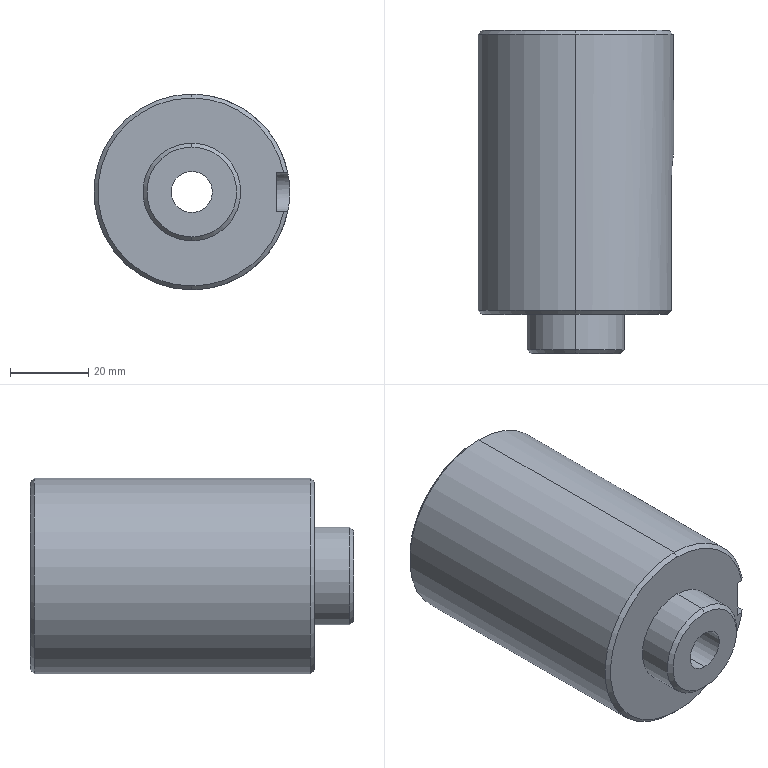Part | SolidWorks | features BaseBody 1 | 1 solid | 29 faces | box 50 x 82.5 x 50 mm | volume 104437 mm3 | cylinder 11 | cone 11 | plane 7 | commonest cylinder face diameters 10.5 x2 25 x2 27.651 x2 28.4 x2 50 x2 10 x1
STEP:
#1=CARTESIAN_POINT('',(0.,71.5,-25.));
#2=VERTEX_POINT('',#1);
#3=CARTESIAN_POINT('',(0.,71.5,25.));
#4=VERTEX_POINT('',#3);
#5=CARTESIAN_POINT('',(0.,71.5,0.));
#6=DIRECTION('',(0.,-1.,0.));
#7=DIRECTION('',(0.,0.,-1.));
#8=AXIS2_PLACEMENT_3D('',#5,#6,#7);
#9=CIRCLE('',#8,25.);
#10=EDGE_CURVE('',#2,#4,#9,.T.);
#11=ORIENTED_EDGE('',*,*,#10,.T.);
#12=CARTESIAN_POINT('',(0.,1.,25.));
#13=VERTEX_POINT('',#12);
#14=CARTESIAN_POINT('',(0.,72.5,25.));
#15=DIRECTION('',(0.,-1.,0.));
#16=VECTOR('',#15,1000.);
#17=LINE('',#14,#16);
#18=EDGE_CURVE('',#4,#13,#17,.T.);
#19=ORIENTED_EDGE('',*,*,#18,.T.);
#20=CARTESIAN_POINT('',(24.495,1.,5.));
#21=VERTEX_POINT('',#20);
#22=CARTESIAN_POINT('',(0.,1.,0.));
#23=DIRECTION('',(0.,1.,0.));
#24=DIRECTION('',(0.,0.,-1.));
#25=AXIS2_PLACEMENT_3D('',#22,#23,#24);
#26=CIRCLE('',#25,25.);
#27=EDGE_CURVE('',#13,#21,#26,.T.);
#28=ORIENTED_EDGE('',*,*,#27,.T.);
#29=CARTESIAN_POINT('',(24.495,36.,5.));
#30=VERTEX_POINT('',#29);
#31=CARTESIAN_POINT('',(24.495,72.5,5.));
#32=DIRECTION('',(0.,1.,0.));
#33=VECTOR('',#32,1000.);
#34=LINE('',#31,#33);
#35=EDGE_CURVE('',#21,#30,#34,.T.);
#36=ORIENTED_EDGE('',*,*,#35,.T.);
#37=CARTESIAN_POINT('',(24.495,36.,-5.));
#38=VERTEX_POINT('',#37);
#39=CARTESIAN_POINT('',(24.495,36.,5.));
#40=CARTESIAN_POINT('',(24.495,36.331,5.));
#41=CARTESIAN_POINT('',(24.502,36.657,4.967));
#42=CARTESIAN_POINT('',(24.527,37.297,4.84));
#43=CARTESIAN_POINT('',(24.546,37.615,4.743));
#44=CARTESIAN_POINT('',(24.593,38.22,4.492));
#45=CARTESIAN_POINT('',(24.621,38.506,4.339));
#46=CARTESIAN_POINT('',(24.682,39.049,3.976));
#47=CARTESIAN_POINT('',(24.716,39.306,3.765));
#48=CARTESIAN_POINT('',(24.782,39.766,3.306));
#49=CARTESIAN_POINT('',(24.814,39.972,3.054));
#50=CARTESIAN_POINT('',(24.875,40.338,2.508));
#51=CARTESIAN_POINT('',(24.903,40.493,2.219));
#52=CARTESIAN_POINT('',(24.949,40.742,1.618));
#53=CARTESIAN_POINT('',(24.968,40.839,1.302));
#54=CARTESIAN_POINT('',(24.993,40.968,0.6559));
#55=CARTESIAN_POINT('',(25.,41.,0.331));
#56=CARTESIAN_POINT('',(25.,41.,-0.3229));
#57=CARTESIAN_POINT('',(24.993,40.968,-0.6551));
#58=CARTESIAN_POINT('',(24.968,40.84,-1.297));
#59=CARTESIAN_POINT('',(24.95,40.745,-1.609));
#60=CARTESIAN_POINT('',(24.915,40.557,-2.064));
#61=CARTESIAN_POINT('',(24.902,40.486,-2.214));
#62=CARTESIAN_POINT('',(24.875,40.332,-2.502));
#63=CARTESIAN_POINT('',(24.86,40.248,-2.642));
#64=CARTESIAN_POINT('',(24.815,39.977,-3.048));
#65=CARTESIAN_POINT('',(24.782,39.77,-3.301));
#66=CARTESIAN_POINT('',(24.716,39.305,-3.766));
#67=CARTESIAN_POINT('',(24.683,39.054,-3.972));
#68=CARTESIAN_POINT('',(24.622,38.513,-4.335));
#69=CARTESIAN_POINT('',(24.594,38.221,-4.492));
#70=CARTESIAN_POINT('',(24.546,37.617,-4.743));
#71=CARTESIAN_POINT('',(24.528,37.305,-4.838));
#72=CARTESIAN_POINT('',(24.502,36.663,-4.967));
#73=CARTESIAN_POINT('',(24.495,36.331,-5.));
#74=CARTESIAN_POINT('',(24.495,36.,-5.));
#75=B_SPLINE_CURVE_WITH_KNOTS('',3,(#39,#40,#41,#42,#43,#44,#45,#46,#47,#48,#49,#50,#51,#52,#53,#54,#55,#56,#57,#58,#59,#60,#61,#62,#63,#64,#65,#66,#67,#68,#69,#70,#71,#72,#73,#74),.UNSPECIFIED.,.F.,.F.,(4,2,2,2,2,2,2,2,2,2,2,2,2,2,2,2,2,4),(0.,0.0009792,0.001958,0.002938,0.003917,0.004896,0.005875,0.006855,0.007834,0.008813,0.009792,0.01028,0.01077,0.01175,0.01273,0.01371,0.01469,0.01567),.UNSPECIFIED.);
#76=EDGE_CURVE('',#30,#38,#75,.T.);
#77=ORIENTED_EDGE('',*,*,#76,.T.);
#78=CARTESIAN_POINT('',(24.495,1.,-5.));
#79=VERTEX_POINT('',#78);
#80=CARTESIAN_POINT('',(24.495,72.5,-5.));
#81=DIRECTION('',(0.,-1.,0.));
#82=VECTOR('',#81,1000.);
#83=LINE('',#80,#82);
#84=EDGE_CURVE('',#38,#79,#83,.T.);
#85=ORIENTED_EDGE('',*,*,#84,.T.);
#86=CARTESIAN_POINT('',(0.,1.,-25.));
#87=VERTEX_POINT('',#86);
#88=CARTESIAN_POINT('',(0.,1.,0.));
#89=DIRECTION('',(0.,1.,0.));
#90=DIRECTION('',(0.,0.,-1.));
#91=AXIS2_PLACEMENT_3D('',#88,#89,#90);
#92=CIRCLE('',#91,25.);
#93=EDGE_CURVE('',#79,#87,#92,.T.);
#94=ORIENTED_EDGE('',*,*,#93,.T.);
#95=CARTESIAN_POINT('',(0.,72.5,-25.));
#96=DIRECTION('',(0.,-1.,0.));
#97=VECTOR('',#96,1000.);
#98=LINE('',#95,#97);
#99=EDGE_CURVE('',#2,#87,#98,.T.);
#100=ORIENTED_EDGE('',*,*,#99,.F.);
#101=EDGE_LOOP('',(#11,#19,#28,#36,#77,#85,#94,#100));
#102=FACE_OUTER_BOUND('',#101,.T.);
#103=CARTESIAN_POINT('',(0.,72.5,0.));
#104=DIRECTION('',(0.,-1.,0.));
#105=DIRECTION('',(0.,0.,-1.));
#106=AXIS2_PLACEMENT_3D('',#103,#104,#105);
#107=CYLINDRICAL_SURFACE('',#106,25.);
#108=ADVANCED_FACE('',(#102),#107,.T.);
#109=CARTESIAN_POINT('',(23.473,0.,-5.));
#110=VERTEX_POINT('',#109);
#111=CARTESIAN_POINT('',(0.,0.,-24.));
#112=VERTEX_POINT('',#111);
#113=CARTESIAN_POINT('',(0.,0.,0.));
#114=DIRECTION('',(0.,1.,0.));
#115=DIRECTION('',(0.,0.,1.));
#116=AXIS2_PLACEMENT_3D('',#113,#114,#115);
#117=CIRCLE('',#116,24.);
#118=EDGE_CURVE('',#110,#112,#117,.T.);
#119=ORIENTED_EDGE('',*,*,#118,.T.);
#120=CARTESIAN_POINT('',(0.,1.,-25.));
#121=DIRECTION('',(0.,0.7071,-0.7071));
#122=VECTOR('',#121,1000.);
#123=LINE('',#120,#122);
#124=EDGE_CURVE('',#112,#87,#123,.T.);
#125=ORIENTED_EDGE('',*,*,#124,.T.);
#126=ORIENTED_EDGE('',*,*,#93,.F.);
#127=CARTESIAN_POINT('',(24.495,1.,-5.));
#128=CARTESIAN_POINT('',(24.155,0.6665,-5.));
#129=CARTESIAN_POINT('',(23.814,0.3332,-5.));
#130=CARTESIAN_POINT('',(23.473,0.,-5.));
#131=B_SPLINE_CURVE_WITH_KNOTS('',3,(#127,#128,#129,#130),.UNSPECIFIED.,.F.,.F.,(4,4),(0.,0.00143),.UNSPECIFIED.);
#132=EDGE_CURVE('',#79,#110,#131,.T.);
#133=ORIENTED_EDGE('',*,*,#132,.T.);
#134=EDGE_LOOP('',(#119,#125,#126,#133));
#135=FACE_OUTER_BOUND('',#134,.T.);
#136=CARTESIAN_POINT('',(0.,1.,0.));
#137=DIRECTION('',(0.,1.,0.));
#138=DIRECTION('',(0.,0.,1.));
#139=AXIS2_PLACEMENT_3D('',#136,#137,#138);
#140=CONICAL_SURFACE('',#139,25.,0.7854);
#141=ADVANCED_FACE('',(#135),#140,.T.);
#142=ORIENTED_EDGE('',*,*,#124,.F.);
#143=CARTESIAN_POINT('',(0.,0.,24.));
#144=VERTEX_POINT('',#143);
#145=CARTESIAN_POINT('',(0.,0.,0.));
#146=DIRECTION('',(0.,1.,0.));
#147=DIRECTION('',(0.,0.,1.));
#148=AXIS2_PLACEMENT_3D('',#145,#146,#147);
#149=CIRCLE('',#148,24.);
#150=EDGE_CURVE('',#112,#144,#149,.T.);
#151=ORIENTED_EDGE('',*,*,#150,.T.);
#152=CARTESIAN_POINT('',(0.,1.,25.));
#153=DIRECTION('',(0.,0.7071,0.7071));
#154=VECTOR('',#153,1000.);
#155=LINE('',#152,#154);
#156=EDGE_CURVE('',#144,#13,#155,.T.);
#157=ORIENTED_EDGE('',*,*,#156,.T.);
#158=CARTESIAN_POINT('',(0.,1.,0.));
#159=DIRECTION('',(0.,1.,0.));
#160=DIRECTION('',(0.,0.,-1.));
#161=AXIS2_PLACEMENT_3D('',#158,#159,#160);
#162=CIRCLE('',#161,25.);
#163=EDGE_CURVE('',#87,#13,#162,.T.);
#164=ORIENTED_EDGE('',*,*,#163,.F.);
#165=EDGE_LOOP('',(#142,#151,#157,#164));
#166=FACE_OUTER_BOUND('',#165,.T.);
#167=CARTESIAN_POINT('',(0.,1.,0.));
#168=DIRECTION('',(0.,1.,0.));
#169=DIRECTION('',(0.,0.,1.));
#170=AXIS2_PLACEMENT_3D('',#167,#168,#169);
#171=CONICAL_SURFACE('',#170,25.,0.7854);
#172=ADVANCED_FACE('',(#166),#171,.T.);
#173=CARTESIAN_POINT('',(0.,72.5,-24.));
#174=VERTEX_POINT('',#173);
#175=CARTESIAN_POINT('',(0.,72.5,24.));
#176=VERTEX_POINT('',#175);
#177=CARTESIAN_POINT('',(0.,72.5,0.));
#178=DIRECTION('',(0.,-1.,0.));
#179=DIRECTION('',(0.,0.,-1.));
#180=AXIS2_PLACEMENT_3D('',#177,#178,#179);
#181=CIRCLE('',#180,24.);
#182=EDGE_CURVE('',#174,#176,#181,.T.);
#183=ORIENTED_EDGE('',*,*,#182,.T.);
#184=CARTESIAN_POINT('',(0.,71.5,25.));
#185=DIRECTION('',(0.,-0.7071,0.7071));
#186=VECTOR('',#185,1000.);
#187=LINE('',#184,#186);
#188=EDGE_CURVE('',#176,#4,#187,.T.);
#189=ORIENTED_EDGE('',*,*,#188,.T.);
#190=ORIENTED_EDGE('',*,*,#10,.F.);
#191=CARTESIAN_POINT('',(0.,71.5,-25.));
#192=DIRECTION('',(0.,-0.7071,-0.7071));
#193=VECTOR('',#192,1000.);
#194=LINE('',#191,#193);
#195=EDGE_CURVE('',#174,#2,#194,.T.);
#196=ORIENTED_EDGE('',*,*,#195,.F.);
#197=EDGE_LOOP('',(#183,#189,#190,#196));
#198=FACE_OUTER_BOUND('',#197,.T.);
#199=CARTESIAN_POINT('',(0.,71.5,0.));
#200=DIRECTION('',(0.,-1.,0.));
#201=DIRECTION('',(0.,0.,-1.));
#202=AXIS2_PLACEMENT_3D('',#199,#200,#201);
#203=CONICAL_SURFACE('',#202,25.,0.7854);
#204=ADVANCED_FACE('',(#198),#203,.T.);
#205=CARTESIAN_POINT('',(0.,-9.,12.5));
#206=VERTEX_POINT('',#205);
#207=CARTESIAN_POINT('',(0.,-9.,-12.5));
#208=VERTEX_POINT('',#207);
#209=CARTESIAN_POINT('',(0.,-9.,0.));
#210=DIRECTION('',(0.,1.,0.));
#211=DIRECTION('',(0.,0.,1.));
#212=AXIS2_PLACEMENT_3D('',#209,#210,#211);
#213=CIRCLE('',#212,12.5);
#214=EDGE_CURVE('',#206,#208,#213,.T.);
#215=ORIENTED_EDGE('',*,*,#214,.T.);
#216=CARTESIAN_POINT('',(0.,0.,-12.5));
#217=VERTEX_POINT('',#216);
#218=CARTESIAN_POINT('',(0.,-10.,-12.5));
#219=DIRECTION('',(0.,1.,0.));
#220=VECTOR('',#219,1000.);
#221=LINE('',#218,#220);
#222=EDGE_CURVE('',#208,#217,#221,.T.);
#223=ORIENTED_EDGE('',*,*,#222,.T.);
#224=CARTESIAN_POINT('',(0.,0.,12.5));
#225=VERTEX_POINT('',#224);
#226=CARTESIAN_POINT('',(0.,0.,0.));
#227=DIRECTION('',(0.,-1.,0.));
#228=DIRECTION('',(0.,0.,1.));
#229=AXIS2_PLACEMENT_3D('',#226,#227,#228);
#230=CIRCLE('',#229,12.5);
#231=EDGE_CURVE('',#217,#225,#230,.T.);
#232=ORIENTED_EDGE('',*,*,#231,.T.);
#233=CARTESIAN_POINT('',(0.,-10.,12.5));
#234=DIRECTION('',(0.,1.,0.));
#235=VECTOR('',#234,1000.);
#236=LINE('',#233,#235);
#237=EDGE_CURVE('',#206,#225,#236,.T.);
#238=ORIENTED_EDGE('',*,*,#237,.F.);
#239=EDGE_LOOP('',(#215,#223,#232,#238));
#240=FACE_OUTER_BOUND('',#239,.T.);
#241=CARTESIAN_POINT('',(0.,-10.,0.));
#242=DIRECTION('',(0.,1.,0.));
#243=DIRECTION('',(0.,0.,1.));
#244=AXIS2_PLACEMENT_3D('',#241,#242,#243);
#245=CYLINDRICAL_SURFACE('',#244,12.5);
#246=ADVANCED_FACE('',(#240),#245,.T.);
#247=CARTESIAN_POINT('',(14.2,71.5,0.));
#248=VERTEX_POINT('',#247);
#249=CARTESIAN_POINT('',(0.,71.5,-14.2));
#250=VERTEX_POINT('',#249);
#251=CARTESIAN_POINT('',(0.,71.5,0.));
#252=DIRECTION('',(0.,1.,0.));
#253=DIRECTION('',(0.,0.,1.));
#254=AXIS2_PLACEMENT_3D('',#251,#252,#253);
#255=CIRCLE('',#254,14.2);
#256=EDGE_CURVE('',#248,#250,#255,.T.);
#257=ORIENTED_EDGE('',*,*,#256,.F.);
#258=CARTESIAN_POINT('',(15.2,72.5,0.));
#259=VERTEX_POINT('',#258);
#260=CARTESIAN_POINT('',(15.2,72.5,0.));
#261=DIRECTION('',(0.7071,0.7071,0.));
#262=VECTOR('',#261,1000.);
#263=LINE('',#260,#262);
#264=EDGE_CURVE('',#248,#259,#263,.T.);
#265=ORIENTED_EDGE('',*,*,#264,.T.);
#266=CARTESIAN_POINT('',(-15.2,72.5,0.));
#267=VERTEX_POINT('',#266);
#268=CARTESIAN_POINT('',(0.,72.5,0.));
#269=DIRECTION('',(0.,-1.,0.));
#270=DIRECTION('',(-1.,0.,0.));
#271=AXIS2_PLACEMENT_3D('',#268,#269,#270);
#272=CIRCLE('',#271,15.2);
#273=EDGE_CURVE('',#267,#259,#272,.T.);
#274=ORIENTED_EDGE('',*,*,#273,.F.);
#275=CARTESIAN_POINT('',(-14.2,71.5,0.));
#276=VERTEX_POINT('',#275);
#277=CARTESIAN_POINT('',(-15.2,72.5,0.));
#278=DIRECTION('',(-0.7071,0.7071,0.));
#279=VECTOR('',#278,1000.);
#280=LINE('',#277,#279);
#281=EDGE_CURVE('',#276,#267,#280,.T.);
#282=ORIENTED_EDGE('',*,*,#281,.F.);
#283=CARTESIAN_POINT('',(0.,71.5,0.));
#284=DIRECTION('',(0.,1.,0.));
#285=DIRECTION('',(0.,0.,1.));
#286=AXIS2_PLACEMENT_3D('',#283,#284,#285);
#287=CIRCLE('',#286,14.2);
#288=EDGE_CURVE('',#250,#276,#287,.T.);
#289=ORIENTED_EDGE('',*,*,#288,.F.);
#290=EDGE_LOOP('',(#257,#265,#274,#282,#289));
#291=FACE_OUTER_BOUND('',#290,.T.);
#292=CARTESIAN_POINT('',(0.,72.5,0.));
#293=DIRECTION('',(0.,1.,0.));
#294=DIRECTION('',(-1.,0.,0.));
#295=AXIS2_PLACEMENT_3D('',#292,#293,#294);
#296=CONICAL_SURFACE('',#295,15.2,0.7854);
#297=ADVANCED_FACE('',(#291),#296,.F.);
#298=CARTESIAN_POINT('',(0.,-10.,11.5));
#299=VERTEX_POINT('',#298);
#300=CARTESIAN_POINT('',(0.,-10.,-11.5));
#301=VERTEX_POINT('',#300);
#302=CARTESIAN_POINT('',(0.,-10.,0.));
#303=DIRECTION('',(0.,1.,0.));
#304=DIRECTION('',(0.,0.,1.));
#305=AXIS2_PLACEMENT_3D('',#302,#303,#304);
#306=CIRCLE('',#305,11.5);
#307=EDGE_CURVE('',#299,#301,#306,.T.);
#308=ORIENTED_EDGE('',*,*,#307,.T.);
#309=CARTESIAN_POINT('',(0.,-9.,-12.5));
#310=DIRECTION('',(0.,0.7071,-0.7071));
#311=VECTOR('',#310,1000.);
#312=LINE('',#309,#311);
#313=EDGE_CURVE('',#301,#208,#312,.T.);
#314=ORIENTED_EDGE('',*,*,#313,.T.);
#315=ORIENTED_EDGE('',*,*,#214,.F.);
#316=CARTESIAN_POINT('',(0.,-9.,12.5));
#317=DIRECTION('',(0.,0.7071,0.7071));
#318=VECTOR('',#317,1000.);
#319=LINE('',#316,#318);
#320=EDGE_CURVE('',#299,#206,#319,.T.);
#321=ORIENTED_EDGE('',*,*,#320,.F.);
#322=EDGE_LOOP('',(#308,#314,#315,#321));
#323=FACE_OUTER_BOUND('',#322,.T.);
#324=CARTESIAN_POINT('',(0.,-9.,0.));
#325=DIRECTION('',(0.,1.,0.));
#326=DIRECTION('',(0.,0.,1.));
#327=AXIS2_PLACEMENT_3D('',#324,#325,#326);
#328=CONICAL_SURFACE('',#327,12.5,0.7854);
#329=ADVANCED_FACE('',(#323),#328,.T.);
#330=CARTESIAN_POINT('',(0.,12.5,-14.2));
#331=VERTEX_POINT('',#330);
#332=CARTESIAN_POINT('',(0.,12.5,14.2));
#333=VERTEX_POINT('',#332);
#334=CARTESIAN_POINT('',(0.,12.5,0.));
#335=DIRECTION('',(0.,1.,0.));
#336=DIRECTION('',(0.,0.,1.));
#337=AXIS2_PLACEMENT_3D('',#334,#335,#336);
#338=CIRCLE('',#337,14.2);
#339=EDGE_CURVE('',#331,#333,#338,.T.);
#340=ORIENTED_EDGE('',*,*,#339,.F.);
#341=CARTESIAN_POINT('',(0.,12.5,-14.2));
#342=DIRECTION('',(0.,1.,0.));
#343=VECTOR('',#342,1000.);
#344=LINE('',#341,#343);
#345=EDGE_CURVE('',#331,#250,#344,.T.);
#346=ORIENTED_EDGE('',*,*,#345,.T.);
#347=ORIENTED_EDGE('',*,*,#288,.T.);
#348=CARTESIAN_POINT('',(0.,71.5,14.2));
#349=VERTEX_POINT('',#348);
#350=CARTESIAN_POINT('',(0.,71.5,0.));
#351=DIRECTION('',(0.,1.,0.));
#352=DIRECTION('',(0.,0.,1.));
#353=AXIS2_PLACEMENT_3D('',#350,#351,#352);
#354=CIRCLE('',#353,14.2);
#355=EDGE_CURVE('',#276,#349,#354,.T.);
#356=ORIENTED_EDGE('',*,*,#355,.T.);
#357=CARTESIAN_POINT('',(0.,12.5,14.2));
#358=DIRECTION('',(0.,1.,0.));
#359=VECTOR('',#358,1000.);
#360=LINE('',#357,#359);
#361=EDGE_CURVE('',#333,#349,#360,.T.);
#362=ORIENTED_EDGE('',*,*,#361,.F.);
#363=EDGE_LOOP('',(#340,#346,#347,#356,#362));
#364=FACE_OUTER_BOUND('',#363,.T.);
#365=CARTESIAN_POINT('',(0.,12.5,0.));
#366=DIRECTION('',(0.,1.,0.));
#367=DIRECTION('',(0.,0.,1.));
#368=AXIS2_PLACEMENT_3D('',#365,#366,#367);
#369=CYLINDRICAL_SURFACE('',#368,14.2);
#370=ADVANCED_FACE('',(#364),#369,.F.);
#371=CARTESIAN_POINT('',(0.,6.847,5.25));
#372=VERTEX_POINT('',#371);
#373=CARTESIAN_POINT('',(0.,6.847,-5.25));
#374=VERTEX_POINT('',#373);
#375=CARTESIAN_POINT('',(0.,6.847,0.));
#376=DIRECTION('',(0.,-1.,0.));
#377=DIRECTION('',(0.,0.,-1.));
#378=AXIS2_PLACEMENT_3D('',#375,#376,#377);
#379=CIRCLE('',#378,5.25);
#380=EDGE_CURVE('',#372,#374,#379,.T.);
#381=ORIENTED_EDGE('',*,*,#380,.F.);
#382=CARTESIAN_POINT('',(0.,-10.,5.25));
#383=VERTEX_POINT('',#382);
#384=CARTESIAN_POINT('',(0.,72.5,5.25));
#385=DIRECTION('',(0.,-1.,0.));
#386=VECTOR('',#385,1000.);
#387=LINE('',#384,#386);
#388=EDGE_CURVE('',#372,#383,#387,.T.);
#389=ORIENTED_EDGE('',*,*,#388,.T.);
#390=CARTESIAN_POINT('',(0.,-10.,-5.25));
#391=VERTEX_POINT('',#390);
#392=CARTESIAN_POINT('',(0.,-10.,0.));
#393=DIRECTION('',(0.,1.,0.));
#394=DIRECTION('',(0.,0.,-1.));
#395=AXIS2_PLACEMENT_3D('',#392,#393,#394);
#396=CIRCLE('',#395,5.25);
#397=EDGE_CURVE('',#391,#383,#396,.T.);
#398=ORIENTED_EDGE('',*,*,#397,.F.);
#399=CARTESIAN_POINT('',(0.,72.5,-5.25));
#400=DIRECTION('',(0.,-1.,0.));
#401=VECTOR('',#400,1000.);
#402=LINE('',#399,#401);
#403=EDGE_CURVE('',#374,#391,#402,.T.);
#404=ORIENTED_EDGE('',*,*,#403,.F.);
#405=EDGE_LOOP('',(#381,#389,#398,#404));
#406=FACE_OUTER_BOUND('',#405,.T.);
#407=CARTESIAN_POINT('',(0.,72.5,0.));
#408=DIRECTION('',(0.,-1.,0.));
#409=DIRECTION('',(0.,0.,-1.));
#410=AXIS2_PLACEMENT_3D('',#407,#408,#409);
#411=CYLINDRICAL_SURFACE('',#410,5.25);
#412=ADVANCED_FACE('',(#406),#411,.F.);
#413=CARTESIAN_POINT('',(-13.825,12.5,0.));
#414=VERTEX_POINT('',#413);
#415=CARTESIAN_POINT('',(13.825,12.5,0.));
#416=VERTEX_POINT('',#415);
#417=CARTESIAN_POINT('',(0.,12.5,0.));
#418=DIRECTION('',(0.,-1.,0.));
#419=DIRECTION('',(1.,0.,0.));
#420=AXIS2_PLACEMENT_3D('',#417,#418,#419);
#421=CIRCLE('',#420,13.825);
#422=EDGE_CURVE('',#414,#416,#421,.T.);
#423=ORIENTED_EDGE('',*,*,#422,.F.);
#424=CARTESIAN_POINT('',(-13.825,12.,0.));
#425=VERTEX_POINT('',#424);
#426=CARTESIAN_POINT('',(-13.825,3.693,0.));
#427=DIRECTION('',(0.,-1.,0.));
#428=VECTOR('',#427,1000.);
#429=LINE('',#426,#428);
#430=EDGE_CURVE('',#414,#425,#429,.T.);
#431=ORIENTED_EDGE('',*,*,#430,.T.);
#432=CARTESIAN_POINT('',(0.,12.,-13.825));
#433=VERTEX_POINT('',#432);
#434=CARTESIAN_POINT('',(0.,12.,0.));
#435=DIRECTION('',(0.,1.,0.));
#436=DIRECTION('',(1.,0.,0.));
#437=AXIS2_PLACEMENT_3D('',#434,#435,#436);
#438=CIRCLE('',#437,13.825);
#439=EDGE_CURVE('',#433,#425,#438,.T.);
#440=ORIENTED_EDGE('',*,*,#439,.F.);
#441=CARTESIAN_POINT('',(13.825,12.,0.));
#442=VERTEX_POINT('',#441);
#443=CARTESIAN_POINT('',(0.,12.,0.));
#444=DIRECTION('',(0.,1.,0.));
#445=DIRECTION('',(1.,0.,0.));
#446=AXIS2_PLACEMENT_3D('',#443,#444,#445);
#447=CIRCLE('',#446,13.825);
#448=EDGE_CURVE('',#442,#433,#447,.T.);
#449=ORIENTED_EDGE('',*,*,#448,.F.);
#450=CARTESIAN_POINT('',(13.825,3.693,0.));
#451=DIRECTION('',(0.,-1.,0.));
#452=VECTOR('',#451,1000.);
#453=LINE('',#450,#452);
#454=EDGE_CURVE('',#416,#442,#453,.T.);
#455=ORIENTED_EDGE('',*,*,#454,.F.);
#456=EDGE_LOOP('',(#423,#431,#440,#449,#455));
#457=FACE_OUTER_BOUND('',#456,.T.);
#458=CARTESIAN_POINT('',(0.,3.693,0.));
#459=DIRECTION('',(0.,-1.,0.));
#460=DIRECTION('',(1.,0.,0.));
#461=AXIS2_PLACEMENT_3D('',#458,#459,#460);
#462=CYLINDRICAL_SURFACE('',#461,13.825);
#463=ADVANCED_FACE('',(#457),#462,.F.);
#464=ORIENTED_EDGE('',*,*,#380,.T.);
#465=CARTESIAN_POINT('',(0.,12.,-13.825));
#466=DIRECTION('',(0.,0.515,-0.8572));
#467=VECTOR('',#466,1000.);
#468=LINE('',#465,#467);
#469=EDGE_CURVE('',#374,#433,#468,.T.);
#470=ORIENTED_EDGE('',*,*,#469,.T.);
#471=ORIENTED_EDGE('',*,*,#439,.T.);
#472=CARTESIAN_POINT('',(0.,12.,13.825));
#473=VERTEX_POINT('',#472);
#474=CARTESIAN_POINT('',(0.,12.,0.));
#475=DIRECTION('',(0.,1.,0.));
#476=DIRECTION('',(1.,0.,0.));
#477=AXIS2_PLACEMENT_3D('',#474,#475,#476);
#478=CIRCLE('',#477,13.825);
#479=EDGE_CURVE('',#425,#473,#478,.T.);
#480=ORIENTED_EDGE('',*,*,#479,.T.);
#481=CARTESIAN_POINT('',(0.,12.,13.825));
#482=DIRECTION('',(0.,0.515,0.8572));
#483=VECTOR('',#482,1000.);
#484=LINE('',#481,#483);
#485=EDGE_CURVE('',#372,#473,#484,.T.);
#486=ORIENTED_EDGE('',*,*,#485,.F.);
#487=EDGE_LOOP('',(#464,#470,#471,#480,#486));
#488=FACE_OUTER_BOUND('',#487,.T.);
#489=CARTESIAN_POINT('',(0.,12.,0.));
#490=DIRECTION('',(0.,1.,0.));
#491=DIRECTION('',(0.,0.,1.));
#492=AXIS2_PLACEMENT_3D('',#489,#490,#491);
#493=CONICAL_SURFACE('',#492,13.825,1.03);
#494=ADVANCED_FACE('',(#488),#493,.F.);
#495=ORIENTED_EDGE('',*,*,#18,.F.);
#496=CARTESIAN_POINT('',(0.,71.5,0.));
#497=DIRECTION('',(0.,-1.,0.));
#498=DIRECTION('',(0.,0.,-1.));
#499=AXIS2_PLACEMENT_3D('',#496,#497,#498);
#500=CIRCLE('',#499,25.);
#501=EDGE_CURVE('',#4,#2,#500,.T.);
#502=ORIENTED_EDGE('',*,*,#501,.T.);
#503=ORIENTED_EDGE('',*,*,#99,.T.);
#504=ORIENTED_EDGE('',*,*,#163,.T.);
#505=EDGE_LOOP('',(#495,#502,#503,#504));
#506=FACE_OUTER_BOUND('',#505,.T.);
#507=CARTESIAN_POINT('',(0.,72.5,0.));
#508=DIRECTION('',(0.,-1.,0.));
#509=DIRECTION('',(0.,0.,-1.));
#510=AXIS2_PLACEMENT_3D('',#507,#508,#509);
#511=CYLINDRICAL_SURFACE('',#510,25.);
#512=ADVANCED_FACE('',(#506),#511,.T.);
#513=ORIENTED_EDGE('',*,*,#156,.F.);
#514=CARTESIAN_POINT('',(23.473,0.,5.));
#515=VERTEX_POINT('',#514);
#516=CARTESIAN_POINT('',(0.,0.,0.));
#517=DIRECTION('',(0.,1.,0.));
#518=DIRECTION('',(0.,0.,1.));
#519=AXIS2_PLACEMENT_3D('',#516,#517,#518);
#520=CIRCLE('',#519,24.);
#521=EDGE_CURVE('',#144,#515,#520,.T.);
#522=ORIENTED_EDGE('',*,*,#521,.T.);
#523=CARTESIAN_POINT('',(23.473,0.,5.));
#524=CARTESIAN_POINT('',(23.814,0.3332,5.));
#525=CARTESIAN_POINT('',(24.155,0.6665,5.));
#526=CARTESIAN_POINT('',(24.495,1.,5.));
#527=B_SPLINE_CURVE_WITH_KNOTS('',3,(#523,#524,#525,#526),.UNSPECIFIED.,.F.,.F.,(4,4),(0.,0.00143),.UNSPECIFIED.);
#528=EDGE_CURVE('',#515,#21,#527,.T.);
#529=ORIENTED_EDGE('',*,*,#528,.T.);
#530=ORIENTED_EDGE('',*,*,#27,.F.);
#531=EDGE_LOOP('',(#513,#522,#529,#530));
#532=FACE_OUTER_BOUND('',#531,.T.);
#533=CARTESIAN_POINT('',(0.,1.,0.));
#534=DIRECTION('',(0.,1.,0.));
#535=DIRECTION('',(0.,0.,1.));
#536=AXIS2_PLACEMENT_3D('',#533,#534,#535);
#537=CONICAL_SURFACE('',#536,25.,0.7854);
#538=ADVANCED_FACE('',(#532),#537,.T.);
#539=ORIENTED_EDGE('',*,*,#188,.F.);
#540=CARTESIAN_POINT('',(0.,72.5,0.));
#541=DIRECTION('',(0.,-1.,0.));
#542=DIRECTION('',(0.,0.,-1.));
#543=AXIS2_PLACEMENT_3D('',#540,#541,#542);
#544=CIRCLE('',#543,24.);
#545=EDGE_CURVE('',#176,#174,#544,.T.);
#546=ORIENTED_EDGE('',*,*,#545,.T.);
#547=ORIENTED_EDGE('',*,*,#195,.T.);
#548=ORIENTED_EDGE('',*,*,#501,.F.);
#549=EDGE_LOOP('',(#539,#546,#547,#548));
#550=FACE_OUTER_BOUND('',#549,.T.);
#551=CARTESIAN_POINT('',(0.,71.5,0.));
#552=DIRECTION('',(0.,-1.,0.));
#553=DIRECTION('',(0.,0.,-1.));
#554=AXIS2_PLACEMENT_3D('',#551,#552,#553);
#555=CONICAL_SURFACE('',#554,25.,0.7854);
#556=ADVANCED_FACE('',(#550),#555,.T.);
#557=CARTESIAN_POINT('',(0.,0.,0.));
#558=DIRECTION('',(0.,-1.,0.));
#559=DIRECTION('',(0.,0.,1.));
#560=AXIS2_PLACEMENT_3D('',#557,#558,#559);
#561=CIRCLE('',#560,12.5);
#562=EDGE_CURVE('',#225,#217,#561,.T.);
#563=ORIENTED_EDGE('',*,*,#562,.F.);
#564=ORIENTED_EDGE('',*,*,#231,.F.);
#565=EDGE_LOOP('',(#563,#564));
#566=FACE_BOUND('',#565,.T.);
#567=ORIENTED_EDGE('',*,*,#118,.F.);
#568=CARTESIAN_POINT('',(21.7,0.,-5.));
#569=VERTEX_POINT('',#568);
#570=CARTESIAN_POINT('',(0.,0.,-5.));
#571=DIRECTION('',(1.,0.,0.));
#572=VECTOR('',#571,1000.);
#573=LINE('',#570,#572);
#574=EDGE_CURVE('',#569,#110,#573,.T.);
#575=ORIENTED_EDGE('',*,*,#574,.F.);
#576=CARTESIAN_POINT('',(21.7,0.,5.));
#577=VERTEX_POINT('',#576);
#578=CARTESIAN_POINT('',(21.7,0.,0.));
#579=DIRECTION('',(0.,0.,-1.));
#580=VECTOR('',#579,1000.);
#581=LINE('',#578,#580);
#582=EDGE_CURVE('',#577,#569,#581,.T.);
#583=ORIENTED_EDGE('',*,*,#582,.F.);
#584=CARTESIAN_POINT('',(0.,0.,5.));
#585=DIRECTION('',(-1.,0.,0.));
#586=VECTOR('',#585,1000.);
#587=LINE('',#584,#586);
#588=EDGE_CURVE('',#515,#577,#587,.T.);
#589=ORIENTED_EDGE('',*,*,#588,.F.);
#590=ORIENTED_EDGE('',*,*,#521,.F.);
#591=ORIENTED_EDGE('',*,*,#150,.F.);
#592=EDGE_LOOP('',(#567,#575,#583,#589,#590,#591));
#593=FACE_OUTER_BOUND('',#592,.T.);
#594=CARTESIAN_POINT('',(0.,0.,0.));
#595=DIRECTION('',(0.,1.,0.));
#596=DIRECTION('',(0.,0.,1.));
#597=AXIS2_PLACEMENT_3D('',#594,#595,#596);
#598=PLANE('',#597);
#599=ADVANCED_FACE('',(#566,#593),#598,.F.);
#600=CARTESIAN_POINT('',(21.7,36.,-5.));
#601=VERTEX_POINT('',#600);
#602=CARTESIAN_POINT('',(21.7,36.,-5.));
#603=DIRECTION('',(0.,1.,0.));
#604=VECTOR('',#603,1000.);
#605=LINE('',#602,#604);
#606=EDGE_CURVE('',#569,#601,#605,.T.);
#607=ORIENTED_EDGE('',*,*,#606,.F.);
#608=ORIENTED_EDGE('',*,*,#574,.T.);
#609=ORIENTED_EDGE('',*,*,#132,.F.);
#610=ORIENTED_EDGE('',*,*,#84,.F.);
#611=CARTESIAN_POINT('',(21.7,36.,-5.));
#612=DIRECTION('',(1.,0.,0.));
#613=VECTOR('',#612,1000.);
#614=LINE('',#611,#613);
#615=EDGE_CURVE('',#601,#38,#614,.T.);
#616=ORIENTED_EDGE('',*,*,#615,.F.);
#617=EDGE_LOOP('',(#607,#608,#609,#610,#616));
#618=FACE_OUTER_BOUND('',#617,.T.);
#619=CARTESIAN_POINT('',(21.7,36.,-5.));
#620=DIRECTION('',(0.,0.,-1.));
#621=DIRECTION('',(0.,1.,0.));
#622=AXIS2_PLACEMENT_3D('',#619,#620,#621);
#623=PLANE('',#622);
#624=ADVANCED_FACE('',(#618),#623,.F.);
#625=CARTESIAN_POINT('',(21.7,36.,5.));
#626=VERTEX_POINT('',#625);
#627=CARTESIAN_POINT('',(21.7,36.,0.));
#628=DIRECTION('',(1.,0.,0.));
#629=DIRECTION('',(0.,0.,-1.));
#630=AXIS2_PLACEMENT_3D('',#627,#628,#629);
#631=CIRCLE('',#630,5.);
#632=EDGE_CURVE('',#601,#626,#631,.T.);
#633=ORIENTED_EDGE('',*,*,#632,.F.);
#634=ORIENTED_EDGE('',*,*,#615,.T.);
#635=ORIENTED_EDGE('',*,*,#76,.F.);
#636=CARTESIAN_POINT('',(21.7,36.,5.));
#637=DIRECTION('',(1.,0.,0.));
#638=VECTOR('',#637,1000.);
#639=LINE('',#636,#638);
#640=EDGE_CURVE('',#626,#30,#639,.T.);
#641=ORIENTED_EDGE('',*,*,#640,.F.);
#642=EDGE_LOOP('',(#633,#634,#635,#641));
#643=FACE_OUTER_BOUND('',#642,.T.);
#644=CARTESIAN_POINT('',(21.7,36.,0.));
#645=DIRECTION('',(1.,0.,0.));
#646=DIRECTION('',(0.,0.,-1.));
#647=AXIS2_PLACEMENT_3D('',#644,#645,#646);
#648=CYLINDRICAL_SURFACE('',#647,5.);
#649=ADVANCED_FACE('',(#643),#648,.F.);
#650=ORIENTED_EDGE('',*,*,#588,.T.);
#651=CARTESIAN_POINT('',(21.7,36.,5.));
#652=DIRECTION('',(0.,-1.,0.));
#653=VECTOR('',#652,1000.);
#654=LINE('',#651,#653);
#655=EDGE_CURVE('',#626,#577,#654,.T.);
#656=ORIENTED_EDGE('',*,*,#655,.F.);
#657=ORIENTED_EDGE('',*,*,#640,.T.);
#658=ORIENTED_EDGE('',*,*,#35,.F.);
#659=ORIENTED_EDGE('',*,*,#528,.F.);
#660=EDGE_LOOP('',(#650,#656,#657,#658,#659));
#661=FACE_OUTER_BOUND('',#660,.T.);
#662=CARTESIAN_POINT('',(21.7,36.,5.));
#663=DIRECTION('',(0.,0.,1.));
#664=DIRECTION('',(0.,-1.,0.));
#665=AXIS2_PLACEMENT_3D('',#662,#663,#664);
#666=PLANE('',#665);
#667=ADVANCED_FACE('',(#661),#666,.F.);
#668=ORIENTED_EDGE('',*,*,#182,.F.);
#669=ORIENTED_EDGE('',*,*,#545,.F.);
#670=EDGE_LOOP('',(#668,#669));
#671=FACE_OUTER_BOUND('',#670,.T.);
#672=ORIENTED_EDGE('',*,*,#273,.T.);
#673=CARTESIAN_POINT('',(0.,72.5,0.));
#674=DIRECTION('',(0.,-1.,0.));
#675=DIRECTION('',(-1.,0.,0.));
#676=AXIS2_PLACEMENT_3D('',#673,#674,#675);
#677=CIRCLE('',#676,15.2);
#678=EDGE_CURVE('',#259,#267,#677,.T.);
#679=ORIENTED_EDGE('',*,*,#678,.T.);
#680=EDGE_LOOP('',(#672,#679));
#681=FACE_BOUND('',#680,.T.);
#682=CARTESIAN_POINT('',(0.,72.5,0.));
#683=DIRECTION('',(0.,1.,0.));
#684=DIRECTION('',(0.,0.,1.));
#685=AXIS2_PLACEMENT_3D('',#682,#683,#684);
#686=PLANE('',#685);
#687=ADVANCED_FACE('',(#671,#681),#686,.T.);
#688=ORIENTED_EDGE('',*,*,#222,.F.);
#689=CARTESIAN_POINT('',(0.,-9.,0.));
#690=DIRECTION('',(0.,1.,0.));
#691=DIRECTION('',(0.,0.,1.));
#692=AXIS2_PLACEMENT_3D('',#689,#690,#691);
#693=CIRCLE('',#692,12.5);
#694=EDGE_CURVE('',#208,#206,#693,.T.);
#695=ORIENTED_EDGE('',*,*,#694,.T.);
#696=ORIENTED_EDGE('',*,*,#237,.T.);
#697=ORIENTED_EDGE('',*,*,#562,.T.);
#698=EDGE_LOOP('',(#688,#695,#696,#697));
#699=FACE_OUTER_BOUND('',#698,.T.);
#700=CARTESIAN_POINT('',(0.,-10.,0.));
#701=DIRECTION('',(0.,1.,0.));
#702=DIRECTION('',(0.,0.,1.));
#703=AXIS2_PLACEMENT_3D('',#700,#701,#702);
#704=CYLINDRICAL_SURFACE('',#703,12.5);
#705=ADVANCED_FACE('',(#699),#704,.T.);
#706=ORIENTED_EDGE('',*,*,#632,.T.);
#707=ORIENTED_EDGE('',*,*,#655,.T.);
#708=ORIENTED_EDGE('',*,*,#582,.T.);
#709=ORIENTED_EDGE('',*,*,#606,.T.);
#710=EDGE_LOOP('',(#706,#707,#708,#709));
#711=FACE_OUTER_BOUND('',#710,.T.);
#712=CARTESIAN_POINT('',(21.7,36.,0.));
#713=DIRECTION('',(1.,0.,0.));
#714=DIRECTION('',(0.,0.,-1.));
#715=AXIS2_PLACEMENT_3D('',#712,#713,#714);
#716=PLANE('',#715);
#717=ADVANCED_FACE('',(#711),#716,.T.);
#718=ORIENTED_EDGE('',*,*,#264,.F.);
#719=CARTESIAN_POINT('',(0.,71.5,0.));
#720=DIRECTION('',(0.,1.,0.));
#721=DIRECTION('',(0.,0.,1.));
#722=AXIS2_PLACEMENT_3D('',#719,#720,#721);
#723=CIRCLE('',#722,14.2);
#724=EDGE_CURVE('',#349,#248,#723,.T.);
#725=ORIENTED_EDGE('',*,*,#724,.F.);
#726=ORIENTED_EDGE('',*,*,#355,.F.);
#727=ORIENTED_EDGE('',*,*,#281,.T.);
#728=ORIENTED_EDGE('',*,*,#678,.F.);
#729=EDGE_LOOP('',(#718,#725,#726,#727,#728));
#730=FACE_OUTER_BOUND('',#729,.T.);
#731=CARTESIAN_POINT('',(0.,72.5,0.));
#732=DIRECTION('',(0.,1.,0.));
#733=DIRECTION('',(-1.,0.,0.));
#734=AXIS2_PLACEMENT_3D('',#731,#732,#733);
#735=CONICAL_SURFACE('',#734,15.2,0.7854);
#736=ADVANCED_FACE('',(#730),#735,.F.);
#737=ORIENTED_EDGE('',*,*,#313,.F.);
#738=CARTESIAN_POINT('',(0.,-10.,0.));
#739=DIRECTION('',(0.,1.,0.));
#740=DIRECTION('',(0.,0.,1.));
#741=AXIS2_PLACEMENT_3D('',#738,#739,#740);
#742=CIRCLE('',#741,11.5);
#743=EDGE_CURVE('',#301,#299,#742,.T.);
#744=ORIENTED_EDGE('',*,*,#743,.T.);
#745=ORIENTED_EDGE('',*,*,#320,.T.);
#746=ORIENTED_EDGE('',*,*,#694,.F.);
#747=EDGE_LOOP('',(#737,#744,#745,#746));
#748=FACE_OUTER_BOUND('',#747,.T.);
#749=CARTESIAN_POINT('',(0.,-9.,0.));
#750=DIRECTION('',(0.,1.,0.));
#751=DIRECTION('',(0.,0.,1.));
#752=AXIS2_PLACEMENT_3D('',#749,#750,#751);
#753=CONICAL_SURFACE('',#752,12.5,0.7854);
#754=ADVANCED_FACE('',(#748),#753,.T.);
#755=ORIENTED_EDGE('',*,*,#345,.F.);
#756=CARTESIAN_POINT('',(0.,12.5,0.));
#757=DIRECTION('',(0.,1.,0.));
#758=DIRECTION('',(0.,0.,1.));
#759=AXIS2_PLACEMENT_3D('',#756,#757,#758);
#760=CIRCLE('',#759,14.2);
#761=EDGE_CURVE('',#333,#331,#760,.T.);
#762=ORIENTED_EDGE('',*,*,#761,.F.);
#763=ORIENTED_EDGE('',*,*,#361,.T.);
#764=ORIENTED_EDGE('',*,*,#724,.T.);
#765=ORIENTED_EDGE('',*,*,#256,.T.);
#766=EDGE_LOOP('',(#755,#762,#763,#764,#765));
#767=FACE_OUTER_BOUND('',#766,.T.);
#768=CARTESIAN_POINT('',(0.,12.5,0.));
#769=DIRECTION('',(0.,1.,0.));
#770=DIRECTION('',(0.,0.,1.));
#771=AXIS2_PLACEMENT_3D('',#768,#769,#770);
#772=CYLINDRICAL_SURFACE('',#771,14.2);
#773=ADVANCED_FACE('',(#767),#772,.F.);
#774=ORIENTED_EDGE('',*,*,#397,.T.);
#775=CARTESIAN_POINT('',(0.,-10.,0.));
#776=DIRECTION('',(0.,1.,0.));
#777=DIRECTION('',(0.,0.,-1.));
#778=AXIS2_PLACEMENT_3D('',#775,#776,#777);
#779=CIRCLE('',#778,5.25);
#780=EDGE_CURVE('',#383,#391,#779,.T.);
#781=ORIENTED_EDGE('',*,*,#780,.T.);
#782=EDGE_LOOP('',(#774,#781));
#783=FACE_BOUND('',#782,.T.);
#784=ORIENTED_EDGE('',*,*,#307,.F.);
#785=ORIENTED_EDGE('',*,*,#743,.F.);
#786=EDGE_LOOP('',(#784,#785));
#787=FACE_OUTER_BOUND('',#786,.T.);
#788=CARTESIAN_POINT('',(0.,-10.,0.));
#789=DIRECTION('',(0.,-1.,0.));
#790=DIRECTION('',(0.,0.,-1.));
#791=AXIS2_PLACEMENT_3D('',#788,#789,#790);
#792=PLANE('',#791);
#793=ADVANCED_FACE('',(#783,#787),#792,.T.);
#794=ORIENTED_EDGE('',*,*,#761,.T.);
#795=ORIENTED_EDGE('',*,*,#339,.T.);
#796=EDGE_LOOP('',(#794,#795));
#797=FACE_OUTER_BOUND('',#796,.T.);
#798=CARTESIAN_POINT('',(0.,12.5,0.));
#799=DIRECTION('',(0.,-1.,0.));
#800=DIRECTION('',(1.,0.,0.));
#801=AXIS2_PLACEMENT_3D('',#798,#799,#800);
#802=CIRCLE('',#801,13.825);
#803=EDGE_CURVE('',#416,#414,#802,.T.);
#804=ORIENTED_EDGE('',*,*,#803,.T.);
#805=ORIENTED_EDGE('',*,*,#422,.T.);
#806=EDGE_LOOP('',(#804,#805));
#807=FACE_BOUND('',#806,.T.);
#808=CARTESIAN_POINT('',(0.,12.5,0.));
#809=DIRECTION('',(0.,1.,0.));
#810=DIRECTION('',(0.,0.,1.));
#811=AXIS2_PLACEMENT_3D('',#808,#809,#810);
#812=PLANE('',#811);
#813=ADVANCED_FACE('',(#797,#807),#812,.T.);
#814=ORIENTED_EDGE('',*,*,#388,.F.);
#815=CARTESIAN_POINT('',(0.,6.847,0.));
#816=DIRECTION('',(0.,-1.,0.));
#817=DIRECTION('',(0.,0.,-1.));
#818=AXIS2_PLACEMENT_3D('',#815,#816,#817);
#819=CIRCLE('',#818,5.25);
#820=EDGE_CURVE('',#374,#372,#819,.T.);
#821=ORIENTED_EDGE('',*,*,#820,.F.);
#822=ORIENTED_EDGE('',*,*,#403,.T.);
#823=ORIENTED_EDGE('',*,*,#780,.F.);
#824=EDGE_LOOP('',(#814,#821,#822,#823));
#825=FACE_OUTER_BOUND('',#824,.T.);
#826=CARTESIAN_POINT('',(0.,72.5,0.));
#827=DIRECTION('',(0.,-1.,0.));
#828=DIRECTION('',(0.,0.,-1.));
#829=AXIS2_PLACEMENT_3D('',#826,#827,#828);
#830=CYLINDRICAL_SURFACE('',#829,5.25);
#831=ADVANCED_FACE('',(#825),#830,.F.);
#832=ORIENTED_EDGE('',*,*,#430,.F.);
#833=ORIENTED_EDGE('',*,*,#803,.F.);
#834=ORIENTED_EDGE('',*,*,#454,.T.);
#835=CARTESIAN_POINT('',(0.,12.,0.));
#836=DIRECTION('',(0.,1.,0.));
#837=DIRECTION('',(1.,0.,0.));
#838=AXIS2_PLACEMENT_3D('',#835,#836,#837);
#839=CIRCLE('',#838,13.825);
#840=EDGE_CURVE('',#473,#442,#839,.T.);
#841=ORIENTED_EDGE('',*,*,#840,.F.);
#842=ORIENTED_EDGE('',*,*,#479,.F.);
#843=EDGE_LOOP('',(#832,#833,#834,#841,#842));
#844=FACE_OUTER_BOUND('',#843,.T.);
#845=CARTESIAN_POINT('',(0.,3.693,0.));
#846=DIRECTION('',(0.,-1.,0.));
#847=DIRECTION('',(1.,0.,0.));
#848=AXIS2_PLACEMENT_3D('',#845,#846,#847);
#849=CYLINDRICAL_SURFACE('',#848,13.825);
#850=ADVANCED_FACE('',(#844),#849,.F.);
#851=ORIENTED_EDGE('',*,*,#469,.F.);
#852=ORIENTED_EDGE('',*,*,#820,.T.);
#853=ORIENTED_EDGE('',*,*,#485,.T.);
#854=ORIENTED_EDGE('',*,*,#840,.T.);
#855=ORIENTED_EDGE('',*,*,#448,.T.);
#856=EDGE_LOOP('',(#851,#852,#853,#854,#855));
#857=FACE_OUTER_BOUND('',#856,.T.);
#858=CARTESIAN_POINT('',(0.,12.,0.));
#859=DIRECTION('',(0.,1.,0.));
#860=DIRECTION('',(0.,0.,1.));
#861=AXIS2_PLACEMENT_3D('',#858,#859,#860);
#862=CONICAL_SURFACE('',#861,13.825,1.03);
#863=ADVANCED_FACE('',(#857),#862,.F.);
#864=CLOSED_SHELL('',(#108,#141,#172,#204,#246,#297,#329,#370,#412,#463,#494,#512,#538,#556,#599,#624,#649,#667,#687,#705,#717,#736,#754,#773,#793,#813,#831,#850,#863));
#865=MANIFOLD_SOLID_BREP('',#864);
#866=CARTESIAN_POINT('',(0.,0.,0.));
#867=DIRECTION('',(0.,0.,1.));
#868=DIRECTION('',(1.,0.,0.));
#869=AXIS2_PLACEMENT_3D('',#866,#867,#868);
#870=(LENGTH_UNIT()NAMED_UNIT(*)SI_UNIT(.MILLI.,.METRE.));
#871=UNCERTAINTY_MEASURE_WITH_UNIT(LENGTH_MEASURE(0.00001),#870,'','');
#872=(NAMED_UNIT(*)PLANE_ANGLE_UNIT()SI_UNIT($,.RADIAN.));
#873=(NAMED_UNIT(*)SI_UNIT($,.STERADIAN.)SOLID_ANGLE_UNIT());
#874=(GEOMETRIC_REPRESENTATION_CONTEXT(3)GLOBAL_UNCERTAINTY_ASSIGNED_CONTEXT((#871))GLOBAL_UNIT_ASSIGNED_CONTEXT((#870,#872,#873))REPRESENTATION_CONTEXT('',''));
#875=ADVANCED_BREP_SHAPE_REPRESENTATION('',(#865,#869),#874);